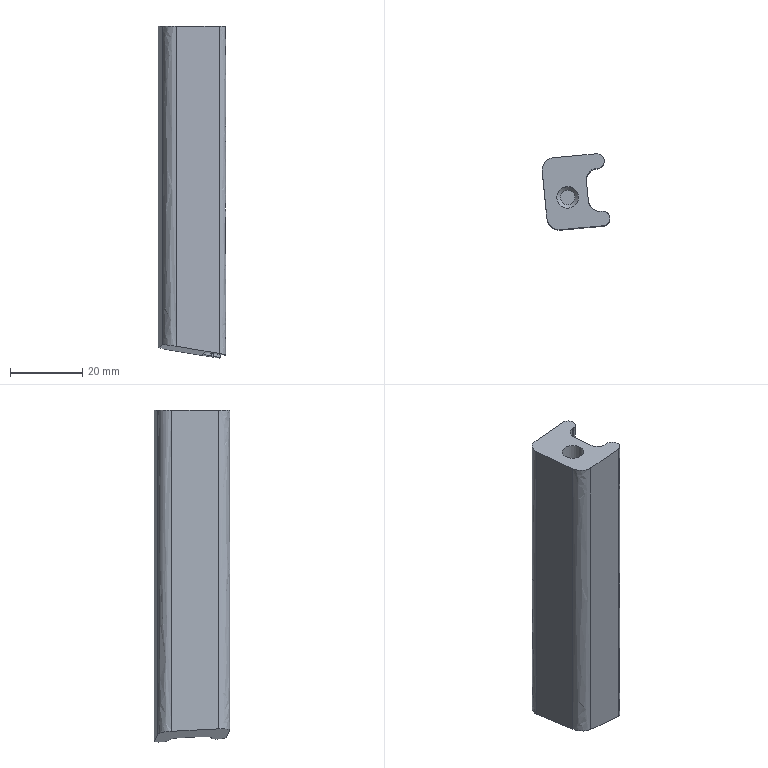Part | NX | features solid 2 | 1 solid | 17 faces | box 18.726 x 21.054 x 92.036 mm | volume 24328 mm3 | plane 8 | spline 7 | cone 1 | cylinder 1 | commonest cylinder face diameters 6 x1
STEP:
#1=CARTESIAN_POINT('',(867.968,-152.567,138.));
#2=VERTEX_POINT('',#1);
#3=CARTESIAN_POINT('',(870.968,-152.567,138.));
#4=DIRECTION('',(0.,0.,-1.));
#5=DIRECTION('',(-1.,0.,0.));
#6=AXIS2_PLACEMENT_3D('',#3,#4,#5);
#7=CIRCLE('',#6,3.);
#8=EDGE_CURVE('',#2,#2,#7,.T.);
#9=ORIENTED_EDGE('',*,*,#8,.T.);
#10=EDGE_LOOP('',(#9));
#11=FACE_BOUND('',#10,.T.);
#12=CARTESIAN_POINT('',(876.165,-147.805,138.));
#13=VERTEX_POINT('',#12);
#14=CARTESIAN_POINT('',(878.77,-144.615,138.));
#15=VERTEX_POINT('',#14);
#16=CARTESIAN_POINT('',(879.063,-147.547,138.));
#17=DIRECTION('',(0.,0.,-1.));
#18=DIRECTION('',(0.3864,-0.9223,0.));
#19=AXIS2_PLACEMENT_3D('',#16,#17,#18);
#20=ELLIPSE('',#19,2.95,2.906);
#21=EDGE_CURVE('',#13,#15,#20,.T.);
#22=ORIENTED_EDGE('',*,*,#21,.T.);
#23=CARTESIAN_POINT('',(879.272,-144.569,138.));
#24=VERTEX_POINT('',#23);
#25=CARTESIAN_POINT('',(879.272,-144.569,138.));
#26=DIRECTION('',(-0.9958,-0.09106,0.));
#27=VECTOR('',#26,1000.);
#28=LINE('',#25,#27);
#29=EDGE_CURVE('',#24,#15,#28,.T.);
#30=ORIENTED_EDGE('',*,*,#29,.F.);
#31=CARTESIAN_POINT('',(878.865,-140.495,138.));
#32=VERTEX_POINT('',#31);
#33=CARTESIAN_POINT('',(879.068,-142.532,138.));
#34=DIRECTION('',(0.,0.,-1.));
#35=DIRECTION('',(0.3864,-0.9223,0.));
#36=AXIS2_PLACEMENT_3D('',#33,#34,#35);
#37=ELLIPSE('',#36,2.05,2.02);
#38=EDGE_CURVE('',#32,#24,#37,.T.);
#39=ORIENTED_EDGE('',*,*,#38,.F.);
#40=CARTESIAN_POINT('',(867.073,-141.573,138.));
#41=VERTEX_POINT('',#40);
#42=CARTESIAN_POINT('',(878.865,-140.495,138.));
#43=DIRECTION('',(-0.9958,-0.09106,0.));
#44=VECTOR('',#43,1000.);
#45=LINE('',#42,#44);
#46=EDGE_CURVE('',#32,#41,#45,.T.);
#47=ORIENTED_EDGE('',*,*,#46,.T.);
#48=CARTESIAN_POINT('',(863.937,-145.412,138.));
#49=VERTEX_POINT('',#48);
#50=CARTESIAN_POINT('',(867.426,-145.101,138.));
#51=DIRECTION('',(0.,0.,-1.));
#52=DIRECTION('',(0.3864,-0.9223,0.));
#53=AXIS2_PLACEMENT_3D('',#50,#51,#52);
#54=ELLIPSE('',#53,3.55,3.497);
#55=EDGE_CURVE('',#49,#41,#54,.T.);
#56=ORIENTED_EDGE('',*,*,#55,.F.);
#57=CARTESIAN_POINT('',(865.2,-158.31,138.));
#58=VERTEX_POINT('',#57);
#59=CARTESIAN_POINT('',(865.2,-158.31,138.));
#60=DIRECTION('',(-0.09741,0.9952,0.));
#61=VECTOR('',#60,1000.);
#62=LINE('',#59,#61);
#63=EDGE_CURVE('',#58,#49,#62,.T.);
#64=ORIENTED_EDGE('',*,*,#63,.F.);
#65=CARTESIAN_POINT('',(869.041,-161.526,138.));
#66=VERTEX_POINT('',#65);
#67=CARTESIAN_POINT('',(868.688,-157.998,138.));
#68=DIRECTION('',(0.,0.,-1.));
#69=DIRECTION('',(0.3864,-0.9223,0.));
#70=AXIS2_PLACEMENT_3D('',#67,#68,#69);
#71=ELLIPSE('',#70,3.55,3.497);
#72=EDGE_CURVE('',#66,#58,#71,.T.);
#73=ORIENTED_EDGE('',*,*,#72,.F.);
#74=CARTESIAN_POINT('',(880.826,-160.449,138.));
#75=VERTEX_POINT('',#74);
#76=CARTESIAN_POINT('',(880.826,-160.449,138.));
#77=DIRECTION('',(-0.9958,-0.09106,0.));
#78=VECTOR('',#77,1000.);
#79=LINE('',#76,#78);
#80=EDGE_CURVE('',#75,#66,#79,.T.);
#81=ORIENTED_EDGE('',*,*,#80,.F.);
#82=CARTESIAN_POINT('',(880.419,-156.374,138.));
#83=VERTEX_POINT('',#82);
#84=CARTESIAN_POINT('',(880.622,-158.411,138.));
#85=DIRECTION('',(0.,0.,-1.));
#86=DIRECTION('',(0.3864,-0.9223,0.));
#87=AXIS2_PLACEMENT_3D('',#84,#85,#86);
#88=ELLIPSE('',#87,2.05,2.02);
#89=EDGE_CURVE('',#83,#75,#88,.T.);
#90=ORIENTED_EDGE('',*,*,#89,.F.);
#91=CARTESIAN_POINT('',(879.938,-156.418,138.));
#92=VERTEX_POINT('',#91);
#93=CARTESIAN_POINT('',(880.419,-156.374,138.));
#94=DIRECTION('',(-0.9958,-0.09106,0.));
#95=VECTOR('',#94,1000.);
#96=LINE('',#93,#95);
#97=EDGE_CURVE('',#83,#92,#96,.T.);
#98=ORIENTED_EDGE('',*,*,#97,.T.);
#99=CARTESIAN_POINT('',(876.746,-153.745,138.));
#100=VERTEX_POINT('',#99);
#101=CARTESIAN_POINT('',(879.645,-153.487,138.));
#102=DIRECTION('',(0.,0.,-1.));
#103=DIRECTION('',(0.3864,-0.9223,0.));
#104=AXIS2_PLACEMENT_3D('',#101,#102,#103);
#105=ELLIPSE('',#104,2.95,2.906);
#106=EDGE_CURVE('',#92,#100,#105,.T.);
#107=ORIENTED_EDGE('',*,*,#106,.T.);
#108=CARTESIAN_POINT('',(876.746,-153.745,138.));
#109=DIRECTION('',(-0.09741,0.9952,0.));
#110=VECTOR('',#109,1000.);
#111=LINE('',#108,#110);
#112=EDGE_CURVE('',#100,#13,#111,.T.);
#113=ORIENTED_EDGE('',*,*,#112,.T.);
#114=EDGE_LOOP('',(#22,#30,#39,#47,#56,#64,#73,#81,#90,#98,#107,#113));
#115=FACE_BOUND('',#114,.T.);
#116=CARTESIAN_POINT('',(855.864,-126.307,138.));
#117=DIRECTION('',(0.,0.,1.));
#118=DIRECTION('',(-1.,0.,0.));
#119=AXIS2_PLACEMENT_3D('',#116,#117,#118);
#120=PLANE('',#119);
#121=ADVANCED_FACE('',(#11,#115),#120,.T.);
#122=CARTESIAN_POINT('',(876.165,-147.805,47.137));
#123=VERTEX_POINT('',#122);
#124=CARTESIAN_POINT('',(878.77,-144.615,46.503));
#125=VERTEX_POINT('',#124);
#126=CARTESIAN_POINT('',(876.165,-147.805,47.137));
#127=CARTESIAN_POINT('',(876.089,-147.032,47.097));
#128=CARTESIAN_POINT('',(876.569,-145.46,46.914));
#129=CARTESIAN_POINT('',(878.006,-144.685,46.631));
#130=CARTESIAN_POINT('',(878.77,-144.615,46.503));
#131=B_SPLINE_CURVE_WITH_KNOTS('',3,(#126,#127,#128,#129,#130),.UNSPECIFIED.,.F.,.F.,(4,1,4),(0.,0.002301,0.004602),.UNSPECIFIED.);
#132=EDGE_CURVE('',#123,#125,#131,.T.);
#133=ORIENTED_EDGE('',*,*,#132,.F.);
#134=CARTESIAN_POINT('',(876.746,-153.745,47.443));
#135=VERTEX_POINT('',#134);
#136=CARTESIAN_POINT('',(876.746,-153.745,47.443));
#137=CARTESIAN_POINT('',(876.552,-151.765,47.341));
#138=CARTESIAN_POINT('',(876.359,-149.785,47.239));
#139=CARTESIAN_POINT('',(876.165,-147.805,47.137));
#140=B_SPLINE_CURVE_WITH_KNOTS('',3,(#136,#137,#138,#139),.UNSPECIFIED.,.F.,.F.,(4,4),(0.,0.005976),.UNSPECIFIED.);
#141=EDGE_CURVE('',#135,#123,#140,.T.);
#142=ORIENTED_EDGE('',*,*,#141,.F.);
#143=CARTESIAN_POINT('',(879.938,-156.418,47.11));
#144=VERTEX_POINT('',#143);
#145=CARTESIAN_POINT('',(879.938,-156.418,47.11));
#146=CARTESIAN_POINT('',(879.172,-156.488,47.238));
#147=CARTESIAN_POINT('',(877.606,-155.987,47.456));
#148=CARTESIAN_POINT('',(876.822,-154.521,47.483));
#149=CARTESIAN_POINT('',(876.746,-153.745,47.443));
#150=B_SPLINE_CURVE_WITH_KNOTS('',3,(#145,#146,#147,#148,#149),.UNSPECIFIED.,.F.,.F.,(4,1,4),(0.,0.002307,0.004615),.UNSPECIFIED.);
#151=EDGE_CURVE('',#144,#135,#150,.T.);
#152=ORIENTED_EDGE('',*,*,#151,.F.);
#153=CARTESIAN_POINT('',(880.419,-156.374,47.03));
#154=VERTEX_POINT('',#153);
#155=CARTESIAN_POINT('',(880.419,-156.374,47.03));
#156=CARTESIAN_POINT('',(880.259,-156.389,47.057));
#157=CARTESIAN_POINT('',(880.098,-156.404,47.083));
#158=CARTESIAN_POINT('',(879.938,-156.418,47.11));
#159=B_SPLINE_CURVE_WITH_KNOTS('',3,(#155,#156,#157,#158),.UNSPECIFIED.,.F.,.F.,(4,4),(0.,0.0004894),.UNSPECIFIED.);
#160=EDGE_CURVE('',#154,#144,#159,.T.);
#161=ORIENTED_EDGE('',*,*,#160,.F.);
#162=CARTESIAN_POINT('',(880.826,-160.449,47.239));
#163=VERTEX_POINT('',#162);
#164=CARTESIAN_POINT('',(880.419,-156.374,47.03));
#165=CARTESIAN_POINT('',(880.951,-156.326,46.941));
#166=CARTESIAN_POINT('',(882.038,-156.672,46.79));
#167=CARTESIAN_POINT('',(882.855,-158.205,46.762));
#168=CARTESIAN_POINT('',(882.359,-159.862,46.953));
#169=CARTESIAN_POINT('',(881.358,-160.4,47.15));
#170=CARTESIAN_POINT('',(880.826,-160.449,47.239));
#171=B_SPLINE_CURVE_WITH_KNOTS('',3,(#164,#165,#166,#167,#168,#169,#170),.UNSPECIFIED.,.F.,.F.,(4,1,1,1,4),(0.,0.001602,0.003204,0.004806,0.006408),.UNSPECIFIED.);
#172=EDGE_CURVE('',#154,#163,#171,.T.);
#173=ORIENTED_EDGE('',*,*,#172,.T.);
#174=CARTESIAN_POINT('',(869.041,-161.526,49.205));
#175=VERTEX_POINT('',#174);
#176=CARTESIAN_POINT('',(880.826,-160.449,47.239));
#177=CARTESIAN_POINT('',(876.898,-160.808,47.894));
#178=CARTESIAN_POINT('',(872.969,-161.167,48.549));
#179=CARTESIAN_POINT('',(869.041,-161.526,49.205));
#180=B_SPLINE_CURVE_WITH_KNOTS('',3,(#176,#177,#178,#179),.UNSPECIFIED.,.F.,.F.,(4,4),(0.,0.012),.UNSPECIFIED.);
#181=EDGE_CURVE('',#163,#175,#180,.T.);
#182=ORIENTED_EDGE('',*,*,#181,.T.);
#183=CARTESIAN_POINT('',(865.2,-158.31,49.605));
#184=VERTEX_POINT('',#183);
#185=CARTESIAN_POINT('',(869.041,-161.526,49.205));
#186=CARTESIAN_POINT('',(868.118,-161.611,49.359));
#187=CARTESIAN_POINT('',(866.234,-161.007,49.621));
#188=CARTESIAN_POINT('',(865.291,-159.243,49.654));
#189=CARTESIAN_POINT('',(865.2,-158.31,49.605));
#190=B_SPLINE_CURVE_WITH_KNOTS('',3,(#185,#186,#187,#188,#189),.UNSPECIFIED.,.F.,.F.,(4,1,4),(0.,0.002777,0.005553),.UNSPECIFIED.);
#191=EDGE_CURVE('',#175,#184,#190,.T.);
#192=ORIENTED_EDGE('',*,*,#191,.T.);
#193=CARTESIAN_POINT('',(863.937,-145.412,48.94));
#194=VERTEX_POINT('',#193);
#195=CARTESIAN_POINT('',(865.2,-158.31,49.605));
#196=CARTESIAN_POINT('',(864.779,-154.011,49.384));
#197=CARTESIAN_POINT('',(864.358,-149.711,49.162));
#198=CARTESIAN_POINT('',(863.937,-145.412,48.94));
#199=B_SPLINE_CURVE_WITH_KNOTS('',3,(#195,#196,#197,#198),.UNSPECIFIED.,.F.,.F.,(4,4),(0.,0.01298),.UNSPECIFIED.);
#200=EDGE_CURVE('',#184,#194,#199,.T.);
#201=ORIENTED_EDGE('',*,*,#200,.T.);
#202=CARTESIAN_POINT('',(867.073,-141.573,48.178));
#203=VERTEX_POINT('',#202);
#204=CARTESIAN_POINT('',(863.937,-145.412,48.94));
#205=CARTESIAN_POINT('',(863.846,-144.482,48.892));
#206=CARTESIAN_POINT('',(864.424,-142.59,48.672));
#207=CARTESIAN_POINT('',(866.153,-141.657,48.332));
#208=CARTESIAN_POINT('',(867.073,-141.573,48.178));
#209=B_SPLINE_CURVE_WITH_KNOTS('',3,(#204,#205,#206,#207,#208),.UNSPECIFIED.,.F.,.F.,(4,1,4),(0.,0.002769,0.005538),.UNSPECIFIED.);
#210=EDGE_CURVE('',#194,#203,#209,.T.);
#211=ORIENTED_EDGE('',*,*,#210,.T.);
#212=CARTESIAN_POINT('',(878.865,-140.495,46.211));
#213=VERTEX_POINT('',#212);
#214=CARTESIAN_POINT('',(878.865,-140.495,46.211));
#215=CARTESIAN_POINT('',(874.934,-140.854,46.867));
#216=CARTESIAN_POINT('',(871.003,-141.214,47.522));
#217=CARTESIAN_POINT('',(867.073,-141.573,48.178));
#218=B_SPLINE_CURVE_WITH_KNOTS('',3,(#214,#215,#216,#217),.UNSPECIFIED.,.F.,.F.,(4,4),(0.,0.012),.UNSPECIFIED.);
#219=EDGE_CURVE('',#213,#203,#218,.T.);
#220=ORIENTED_EDGE('',*,*,#219,.F.);
#221=CARTESIAN_POINT('',(879.272,-144.569,46.42));
#222=VERTEX_POINT('',#221);
#223=CARTESIAN_POINT('',(878.865,-140.495,46.211));
#224=CARTESIAN_POINT('',(879.397,-140.446,46.122));
#225=CARTESIAN_POINT('',(880.484,-140.792,45.971));
#226=CARTESIAN_POINT('',(881.301,-142.326,45.943));
#227=CARTESIAN_POINT('',(880.805,-143.983,46.134));
#228=CARTESIAN_POINT('',(879.804,-144.52,46.331));
#229=CARTESIAN_POINT('',(879.272,-144.569,46.42));
#230=B_SPLINE_CURVE_WITH_KNOTS('',3,(#223,#224,#225,#226,#227,#228,#229),.UNSPECIFIED.,.F.,.F.,(4,1,1,1,4),(0.,0.001602,0.003204,0.004806,0.006408),.UNSPECIFIED.);
#231=EDGE_CURVE('',#213,#222,#230,.T.);
#232=ORIENTED_EDGE('',*,*,#231,.T.);
#233=CARTESIAN_POINT('',(879.272,-144.569,46.42));
#234=CARTESIAN_POINT('',(879.105,-144.584,46.448));
#235=CARTESIAN_POINT('',(878.938,-144.6,46.475));
#236=CARTESIAN_POINT('',(878.77,-144.615,46.503));
#237=B_SPLINE_CURVE_WITH_KNOTS('',3,(#233,#234,#235,#236),.UNSPECIFIED.,.F.,.F.,(4,4),(0.,0.0005105),.UNSPECIFIED.);
#238=EDGE_CURVE('',#222,#125,#237,.T.);
#239=ORIENTED_EDGE('',*,*,#238,.T.);
#240=EDGE_LOOP('',(#133,#142,#152,#161,#173,#182,#192,#201,#211,#220,#232,#239));
#241=FACE_BOUND('',#240,.T.);
#242=CARTESIAN_POINT('',(882.55,-140.343,45.609));
#243=CARTESIAN_POINT('',(882.802,-161.67,47.003));
#244=CARTESIAN_POINT('',(863.732,-140.367,48.634));
#245=CARTESIAN_POINT('',(863.984,-161.694,50.029));
#246=B_SPLINE_SURFACE_WITH_KNOTS('',1,1,((#242,#243),(#244,#245)),.PLANE_SURF.,.F.,.F.,.F.,(2,2),(2,2),(0.2039,0.9074),(0.09274,0.922),.PIECEWISE_BEZIER_KNOTS.);
#247=ADVANCED_FACE('',(#241),#246,.F.);
#248=CARTESIAN_POINT('',(876.746,-153.745,211.));
#249=DIRECTION('',(0.,0.,-1.));
#250=VECTOR('',#249,1000.);
#251=LINE('',#248,#250);
#252=EDGE_CURVE('',#100,#135,#251,.T.);
#253=ORIENTED_EDGE('',*,*,#252,.T.);
#254=ORIENTED_EDGE('',*,*,#141,.T.);
#255=CARTESIAN_POINT('',(876.165,-147.805,211.));
#256=DIRECTION('',(0.,0.,-1.));
#257=VECTOR('',#256,1000.);
#258=LINE('',#255,#257);
#259=EDGE_CURVE('',#13,#123,#258,.T.);
#260=ORIENTED_EDGE('',*,*,#259,.F.);
#261=ORIENTED_EDGE('',*,*,#112,.F.);
#262=EDGE_LOOP('',(#253,#254,#260,#261));
#263=FACE_BOUND('',#262,.T.);
#264=CARTESIAN_POINT('',(876.746,-153.745,211.));
#265=DIRECTION('',(0.9952,0.09741,0.));
#266=DIRECTION('',(0.09741,-0.9952,0.));
#267=AXIS2_PLACEMENT_3D('',#264,#265,#266);
#268=PLANE('',#267);
#269=ADVANCED_FACE('',(#263),#268,.T.);
#270=CARTESIAN_POINT('',(879.938,-156.418,211.));
#271=DIRECTION('',(0.,0.,-1.));
#272=VECTOR('',#271,1000.);
#273=LINE('',#270,#272);
#274=EDGE_CURVE('',#92,#144,#273,.T.);
#275=ORIENTED_EDGE('',*,*,#274,.T.);
#276=ORIENTED_EDGE('',*,*,#151,.T.);
#277=ORIENTED_EDGE('',*,*,#252,.F.);
#278=ORIENTED_EDGE('',*,*,#106,.F.);
#279=EDGE_LOOP('',(#275,#276,#277,#278));
#280=FACE_BOUND('',#279,.T.);
#281=CARTESIAN_POINT('',(879.938,-156.418,138.));
#282=CARTESIAN_POINT('',(879.938,-156.418,46.565));
#283=CARTESIAN_POINT('',(879.174,-156.488,138.));
#284=CARTESIAN_POINT('',(879.174,-156.488,46.565));
#285=CARTESIAN_POINT('',(877.587,-155.982,138.));
#286=CARTESIAN_POINT('',(877.587,-155.982,46.565));
#287=CARTESIAN_POINT('',(876.812,-154.492,138.));
#288=CARTESIAN_POINT('',(876.812,-154.492,46.565));
#289=CARTESIAN_POINT('',(876.744,-153.718,138.));
#290=CARTESIAN_POINT('',(876.744,-153.718,46.565));
#291=B_SPLINE_SURFACE_WITH_KNOTS('',3,1,((#281,#282),(#283,#284),(#285,#286),(#287,#288),(#289,#290)),.SURF_OF_LINEAR_EXTRUSION.,.F.,.F.,.F.,(4,1,4),(2,2),(0.3012,1.092,1.884),(0.,1.),.UNSPECIFIED.);
#292=ADVANCED_FACE('',(#280),#291,.F.);
#293=CARTESIAN_POINT('',(880.419,-156.374,211.));
#294=DIRECTION('',(0.,0.,-1.));
#295=VECTOR('',#294,1000.);
#296=LINE('',#293,#295);
#297=EDGE_CURVE('',#83,#154,#296,.T.);
#298=ORIENTED_EDGE('',*,*,#297,.T.);
#299=ORIENTED_EDGE('',*,*,#160,.T.);
#300=ORIENTED_EDGE('',*,*,#274,.F.);
#301=ORIENTED_EDGE('',*,*,#97,.F.);
#302=EDGE_LOOP('',(#298,#299,#300,#301));
#303=FACE_BOUND('',#302,.T.);
#304=CARTESIAN_POINT('',(880.419,-156.374,211.));
#305=DIRECTION('',(-0.09106,0.9958,0.));
#306=DIRECTION('',(0.9958,0.09106,0.));
#307=AXIS2_PLACEMENT_3D('',#304,#305,#306);
#308=PLANE('',#307);
#309=ADVANCED_FACE('',(#303),#308,.T.);
#310=ORIENTED_EDGE('',*,*,#89,.T.);
#311=CARTESIAN_POINT('',(880.826,-160.449,211.));
#312=DIRECTION('',(0.,0.,-1.));
#313=VECTOR('',#312,1000.);
#314=LINE('',#311,#313);
#315=EDGE_CURVE('',#75,#163,#314,.T.);
#316=ORIENTED_EDGE('',*,*,#315,.T.);
#317=ORIENTED_EDGE('',*,*,#172,.F.);
#318=ORIENTED_EDGE('',*,*,#297,.F.);
#319=EDGE_LOOP('',(#310,#316,#317,#318));
#320=FACE_BOUND('',#319,.T.);
#321=CARTESIAN_POINT('',(880.381,-156.378,138.));
#322=CARTESIAN_POINT('',(880.381,-156.378,46.233));
#323=CARTESIAN_POINT('',(880.91,-156.319,138.));
#324=CARTESIAN_POINT('',(880.91,-156.319,46.233));
#325=CARTESIAN_POINT('',(882.017,-156.648,138.));
#326=CARTESIAN_POINT('',(882.017,-156.648,46.233));
#327=CARTESIAN_POINT('',(882.855,-158.186,138.));
#328=CARTESIAN_POINT('',(882.855,-158.186,46.233));
#329=CARTESIAN_POINT('',(882.368,-159.857,138.));
#330=CARTESIAN_POINT('',(882.368,-159.857,46.233));
#331=CARTESIAN_POINT('',(881.357,-160.4,138.));
#332=CARTESIAN_POINT('',(881.357,-160.4,46.233));
#333=CARTESIAN_POINT('',(880.826,-160.449,138.));
#334=CARTESIAN_POINT('',(880.826,-160.449,46.233));
#335=B_SPLINE_SURFACE_WITH_KNOTS('',3,1,((#321,#322),(#323,#324),(#325,#326),(#327,#328),(#329,#330),(#331,#332),(#333,#334)),.SURF_OF_LINEAR_EXTRUSION.,.F.,.F.,.F.,(4,1,1,1,4),(2,2),(3.424,4.214,5.004,5.794,6.584),(0.,1.),.UNSPECIFIED.);
#336=ADVANCED_FACE('',(#320),#335,.T.);
#337=ORIENTED_EDGE('',*,*,#80,.T.);
#338=CARTESIAN_POINT('',(869.041,-161.526,211.));
#339=DIRECTION('',(0.,0.,-1.));
#340=VECTOR('',#339,1000.);
#341=LINE('',#338,#340);
#342=EDGE_CURVE('',#66,#175,#341,.T.);
#343=ORIENTED_EDGE('',*,*,#342,.T.);
#344=ORIENTED_EDGE('',*,*,#181,.F.);
#345=ORIENTED_EDGE('',*,*,#315,.F.);
#346=EDGE_LOOP('',(#337,#343,#344,#345));
#347=FACE_BOUND('',#346,.T.);
#348=CARTESIAN_POINT('',(880.826,-160.449,211.));
#349=DIRECTION('',(-0.09106,0.9958,0.));
#350=DIRECTION('',(0.9958,0.09106,0.));
#351=AXIS2_PLACEMENT_3D('',#348,#349,#350);
#352=PLANE('',#351);
#353=ADVANCED_FACE('',(#347),#352,.F.);
#354=ORIENTED_EDGE('',*,*,#72,.T.);
#355=CARTESIAN_POINT('',(865.2,-158.31,211.));
#356=DIRECTION('',(0.,0.,-1.));
#357=VECTOR('',#356,1000.);
#358=LINE('',#355,#357);
#359=EDGE_CURVE('',#58,#184,#358,.T.);
#360=ORIENTED_EDGE('',*,*,#359,.T.);
#361=ORIENTED_EDGE('',*,*,#191,.F.);
#362=ORIENTED_EDGE('',*,*,#342,.F.);
#363=EDGE_LOOP('',(#354,#360,#361,#362));
#364=FACE_BOUND('',#363,.T.);
#365=CARTESIAN_POINT('',(869.074,-161.523,138.));
#366=CARTESIAN_POINT('',(869.074,-161.523,48.672));
#367=CARTESIAN_POINT('',(868.155,-161.616,138.));
#368=CARTESIAN_POINT('',(868.155,-161.616,48.672));
#369=CARTESIAN_POINT('',(866.24,-161.025,138.));
#370=CARTESIAN_POINT('',(866.24,-161.025,48.672));
#371=CARTESIAN_POINT('',(865.291,-159.24,138.));
#372=CARTESIAN_POINT('',(865.291,-159.24,48.672));
#373=CARTESIAN_POINT('',(865.2,-158.31,138.));
#374=CARTESIAN_POINT('',(865.2,-158.31,48.672));
#375=B_SPLINE_SURFACE_WITH_KNOTS('',3,1,((#365,#366),(#367,#368),(#369,#370),(#371,#372),(#373,#374)),.SURF_OF_LINEAR_EXTRUSION.,.F.,.F.,.F.,(4,1,4),(2,2),(0.2918,1.083,1.874),(0.,1.),.UNSPECIFIED.);
#376=ADVANCED_FACE('',(#364),#375,.T.);
#377=ORIENTED_EDGE('',*,*,#63,.T.);
#378=CARTESIAN_POINT('',(863.937,-145.412,211.));
#379=DIRECTION('',(0.,0.,-1.));
#380=VECTOR('',#379,1000.);
#381=LINE('',#378,#380);
#382=EDGE_CURVE('',#49,#194,#381,.T.);
#383=ORIENTED_EDGE('',*,*,#382,.T.);
#384=ORIENTED_EDGE('',*,*,#200,.F.);
#385=ORIENTED_EDGE('',*,*,#359,.F.);
#386=EDGE_LOOP('',(#377,#383,#384,#385));
#387=FACE_BOUND('',#386,.T.);
#388=CARTESIAN_POINT('',(865.2,-158.31,211.));
#389=DIRECTION('',(0.9952,0.09741,0.));
#390=DIRECTION('',(0.09741,-0.9952,0.));
#391=AXIS2_PLACEMENT_3D('',#388,#389,#390);
#392=PLANE('',#391);
#393=ADVANCED_FACE('',(#387),#392,.F.);
#394=ORIENTED_EDGE('',*,*,#55,.T.);
#395=CARTESIAN_POINT('',(867.073,-141.573,211.));
#396=DIRECTION('',(0.,0.,-1.));
#397=VECTOR('',#396,1000.);
#398=LINE('',#395,#397);
#399=EDGE_CURVE('',#41,#203,#398,.T.);
#400=ORIENTED_EDGE('',*,*,#399,.T.);
#401=ORIENTED_EDGE('',*,*,#210,.F.);
#402=ORIENTED_EDGE('',*,*,#382,.F.);
#403=EDGE_LOOP('',(#394,#400,#401,#402));
#404=FACE_BOUND('',#403,.T.);
#405=CARTESIAN_POINT('',(863.941,-145.445,138.));
#406=CARTESIAN_POINT('',(863.941,-145.445,47.639));
#407=CARTESIAN_POINT('',(863.841,-144.518,138.));
#408=CARTESIAN_POINT('',(863.841,-144.518,47.639));
#409=CARTESIAN_POINT('',(864.406,-142.596,138.));
#410=CARTESIAN_POINT('',(864.406,-142.596,47.639));
#411=CARTESIAN_POINT('',(866.156,-141.657,138.));
#412=CARTESIAN_POINT('',(866.156,-141.657,47.639));
#413=CARTESIAN_POINT('',(867.073,-141.573,138.));
#414=CARTESIAN_POINT('',(867.073,-141.573,47.639));
#415=B_SPLINE_SURFACE_WITH_KNOTS('',3,1,((#405,#406),(#407,#408),(#409,#410),(#411,#412),(#413,#414)),.SURF_OF_LINEAR_EXTRUSION.,.F.,.F.,.F.,(4,1,4),(2,2),(1.865,2.654,3.443),(0.,1.),.UNSPECIFIED.);
#416=ADVANCED_FACE('',(#404),#415,.T.);
#417=CARTESIAN_POINT('',(878.865,-140.495,211.));
#418=DIRECTION('',(0.,0.,-1.));
#419=VECTOR('',#418,1000.);
#420=LINE('',#417,#419);
#421=EDGE_CURVE('',#32,#213,#420,.T.);
#422=ORIENTED_EDGE('',*,*,#421,.T.);
#423=ORIENTED_EDGE('',*,*,#219,.T.);
#424=ORIENTED_EDGE('',*,*,#399,.F.);
#425=ORIENTED_EDGE('',*,*,#46,.F.);
#426=EDGE_LOOP('',(#422,#423,#424,#425));
#427=FACE_BOUND('',#426,.T.);
#428=CARTESIAN_POINT('',(878.865,-140.495,211.));
#429=DIRECTION('',(-0.09106,0.9958,0.));
#430=DIRECTION('',(0.9958,0.09106,0.));
#431=AXIS2_PLACEMENT_3D('',#428,#429,#430);
#432=PLANE('',#431);
#433=ADVANCED_FACE('',(#427),#432,.T.);
#434=ORIENTED_EDGE('',*,*,#38,.T.);
#435=CARTESIAN_POINT('',(879.272,-144.569,211.));
#436=DIRECTION('',(0.,0.,-1.));
#437=VECTOR('',#436,1000.);
#438=LINE('',#435,#437);
#439=EDGE_CURVE('',#24,#222,#438,.T.);
#440=ORIENTED_EDGE('',*,*,#439,.T.);
#441=ORIENTED_EDGE('',*,*,#231,.F.);
#442=ORIENTED_EDGE('',*,*,#421,.F.);
#443=EDGE_LOOP('',(#434,#440,#441,#442));
#444=FACE_BOUND('',#443,.T.);
#445=CARTESIAN_POINT('',(878.827,-140.499,138.));
#446=CARTESIAN_POINT('',(878.827,-140.499,45.409));
#447=CARTESIAN_POINT('',(879.356,-140.44,138.));
#448=CARTESIAN_POINT('',(879.356,-140.44,45.409));
#449=CARTESIAN_POINT('',(880.463,-140.769,138.));
#450=CARTESIAN_POINT('',(880.463,-140.769,45.409));
#451=CARTESIAN_POINT('',(881.301,-142.306,138.));
#452=CARTESIAN_POINT('',(881.301,-142.306,45.409));
#453=CARTESIAN_POINT('',(880.814,-143.978,138.));
#454=CARTESIAN_POINT('',(880.814,-143.978,45.409));
#455=CARTESIAN_POINT('',(879.802,-144.521,138.));
#456=CARTESIAN_POINT('',(879.802,-144.521,45.409));
#457=CARTESIAN_POINT('',(879.272,-144.569,138.));
#458=CARTESIAN_POINT('',(879.272,-144.569,45.409));
#459=B_SPLINE_SURFACE_WITH_KNOTS('',3,1,((#445,#446),(#447,#448),(#449,#450),(#451,#452),(#453,#454),(#455,#456),(#457,#458)),.SURF_OF_LINEAR_EXTRUSION.,.F.,.F.,.F.,(4,1,1,1,4),(2,2),(3.424,4.214,5.004,5.794,6.584),(0.,1.),.UNSPECIFIED.);
#460=ADVANCED_FACE('',(#444),#459,.T.);
#461=ORIENTED_EDGE('',*,*,#29,.T.);
#462=CARTESIAN_POINT('',(878.77,-144.615,211.));
#463=DIRECTION('',(0.,0.,-1.));
#464=VECTOR('',#463,1000.);
#465=LINE('',#462,#464);
#466=EDGE_CURVE('',#15,#125,#465,.T.);
#467=ORIENTED_EDGE('',*,*,#466,.T.);
#468=ORIENTED_EDGE('',*,*,#238,.F.);
#469=ORIENTED_EDGE('',*,*,#439,.F.);
#470=EDGE_LOOP('',(#461,#467,#468,#469));
#471=FACE_BOUND('',#470,.T.);
#472=CARTESIAN_POINT('',(879.272,-144.569,211.));
#473=DIRECTION('',(-0.09106,0.9958,0.));
#474=DIRECTION('',(0.9958,0.09106,0.));
#475=AXIS2_PLACEMENT_3D('',#472,#473,#474);
#476=PLANE('',#475);
#477=ADVANCED_FACE('',(#471),#476,.F.);
#478=ORIENTED_EDGE('',*,*,#259,.T.);
#479=ORIENTED_EDGE('',*,*,#132,.T.);
#480=ORIENTED_EDGE('',*,*,#466,.F.);
#481=ORIENTED_EDGE('',*,*,#21,.F.);
#482=EDGE_LOOP('',(#478,#479,#480,#481));
#483=FACE_BOUND('',#482,.T.);
#484=CARTESIAN_POINT('',(876.165,-147.805,138.));
#485=CARTESIAN_POINT('',(876.165,-147.805,45.954));
#486=CARTESIAN_POINT('',(876.089,-147.034,138.));
#487=CARTESIAN_POINT('',(876.089,-147.034,45.954));
#488=CARTESIAN_POINT('',(876.573,-145.441,138.));
#489=CARTESIAN_POINT('',(876.573,-145.441,45.954));
#490=CARTESIAN_POINT('',(878.035,-144.675,138.));
#491=CARTESIAN_POINT('',(878.035,-144.675,45.954));
#492=CARTESIAN_POINT('',(878.798,-144.613,138.));
#493=CARTESIAN_POINT('',(878.798,-144.613,45.954));
#494=B_SPLINE_SURFACE_WITH_KNOTS('',3,1,((#484,#485),(#486,#487),(#488,#489),(#490,#491),(#492,#493)),.SURF_OF_LINEAR_EXTRUSION.,.F.,.F.,.F.,(4,1,4),(2,2),(1.874,2.663,3.452),(0.,1.),.UNSPECIFIED.);
#495=ADVANCED_FACE('',(#483),#494,.F.);
#496=CARTESIAN_POINT('',(871.162,-154.557,112.));
#497=VERTEX_POINT('',#496);
#498=CARTESIAN_POINT('',(870.968,-152.567,112.));
#499=DIRECTION('',(0.,0.,1.));
#500=DIRECTION('',(0.09666,-0.9953,0.));
#501=AXIS2_PLACEMENT_3D('',#498,#499,#500);
#502=CIRCLE('',#501,2.);
#503=EDGE_CURVE('',#497,#497,#502,.T.);
#504=ORIENTED_EDGE('',*,*,#503,.T.);
#505=EDGE_LOOP('',(#504));
#506=FACE_BOUND('',#505,.T.);
#507=CARTESIAN_POINT('',(870.968,-152.567,112.));
#508=DIRECTION('',(0.,0.,-1.));
#509=DIRECTION('',(0.09666,-0.9953,0.));
#510=AXIS2_PLACEMENT_3D('',#507,#508,#509);
#511=PLANE('',#510);
#512=ADVANCED_FACE('',(#506),#511,.F.);
#513=ORIENTED_EDGE('',*,*,#503,.F.);
#514=EDGE_LOOP('',(#513));
#515=FACE_BOUND('',#514,.T.);
#516=CARTESIAN_POINT('',(871.258,-155.553,113.));
#517=VERTEX_POINT('',#516);
#518=CARTESIAN_POINT('',(870.968,-152.567,113.));
#519=DIRECTION('',(0.,0.,1.));
#520=DIRECTION('',(0.09666,-0.9953,0.));
#521=AXIS2_PLACEMENT_3D('',#518,#519,#520);
#522=CIRCLE('',#521,3.);
#523=EDGE_CURVE('',#517,#517,#522,.F.);
#524=ORIENTED_EDGE('',*,*,#523,.F.);
#525=EDGE_LOOP('',(#524));
#526=FACE_BOUND('',#525,.T.);
#527=CARTESIAN_POINT('',(870.968,-152.567,113.));
#528=DIRECTION('',(0.,0.,1.));
#529=DIRECTION('',(-0.09666,0.9953,0.));
#530=AXIS2_PLACEMENT_3D('',#527,#528,#529);
#531=CONICAL_SURFACE('',#530,3.,0.7854);
#532=ADVANCED_FACE('',(#515,#526),#531,.F.);
#533=ORIENTED_EDGE('',*,*,#8,.F.);
#534=EDGE_LOOP('',(#533));
#535=FACE_BOUND('',#534,.T.);
#536=ORIENTED_EDGE('',*,*,#523,.T.);
#537=EDGE_LOOP('',(#536));
#538=FACE_BOUND('',#537,.T.);
#539=CARTESIAN_POINT('',(870.968,-152.567,162.));
#540=DIRECTION('',(0.,0.,-1.));
#541=DIRECTION('',(0.09666,-0.9953,0.));
#542=AXIS2_PLACEMENT_3D('',#539,#540,#541);
#543=CYLINDRICAL_SURFACE('',#542,3.);
#544=ADVANCED_FACE('',(#535,#538),#543,.F.);
#545=CLOSED_SHELL('',(#121,#247,#269,#292,#309,#336,#353,#376,#393,#416,#433,#460,#477,#495,#512,#532,#544));
#546=MANIFOLD_SOLID_BREP('',#545);
#547=(LENGTH_UNIT()NAMED_UNIT(*)SI_UNIT(.MILLI.,.METRE.));
#548=UNCERTAINTY_MEASURE_WITH_UNIT(LENGTH_MEASURE(0.0508),#547,'','');
#549=(NAMED_UNIT(*)PLANE_ANGLE_UNIT()SI_UNIT($,.RADIAN.));
#550=(NAMED_UNIT(*)SI_UNIT($,.STERADIAN.)SOLID_ANGLE_UNIT());
#551=(GEOMETRIC_REPRESENTATION_CONTEXT(3)GLOBAL_UNCERTAINTY_ASSIGNED_CONTEXT((#548))GLOBAL_UNIT_ASSIGNED_CONTEXT((#547,#549,#550))REPRESENTATION_CONTEXT('',''));
#552=ADVANCED_BREP_SHAPE_REPRESENTATION('',(#546),#551);